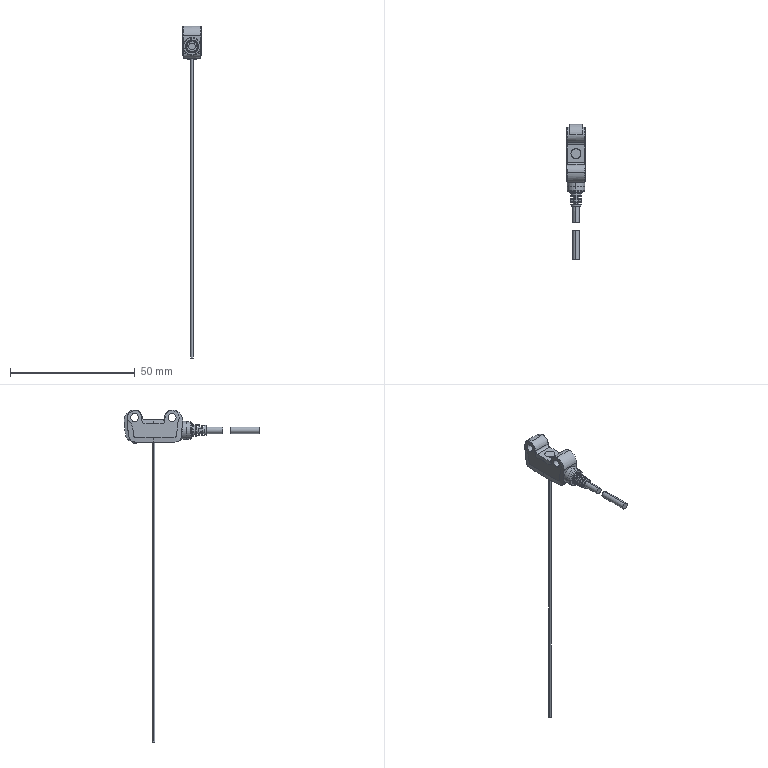Part | NX | features BREP 2 | 2 solids | 287 faces | box 7.512 x 54.319 x 133 mm | volume 2105 mm3 | plane 139 | cylinder 93 | spline 35 | cone 20 | commonest cylinder face diameters 2.6 x11 4 x9 0.5 x6 1 x5 3.2 x4 42.147 x4